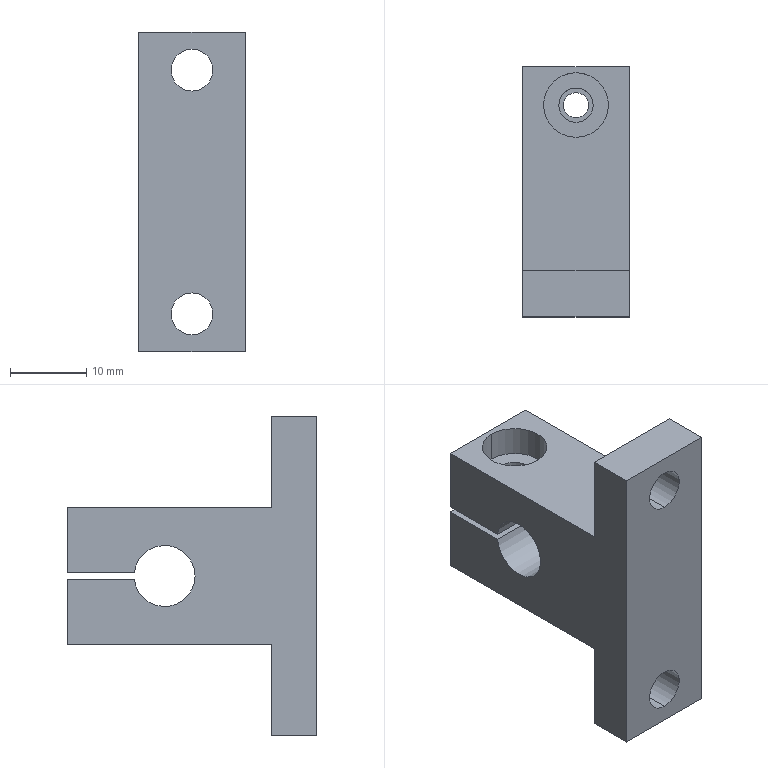Part | STEP file | Φ8 guide shaft seat | 1 solid | 26 faces | box 14 x 32.8 x 42 mm | volume 8820 mm3 | plane 14 | cylinder 12 | commonest cylinder face diameters 5.5 x4 3.3 x2 4.5 x2 8 x2 8.5 x2